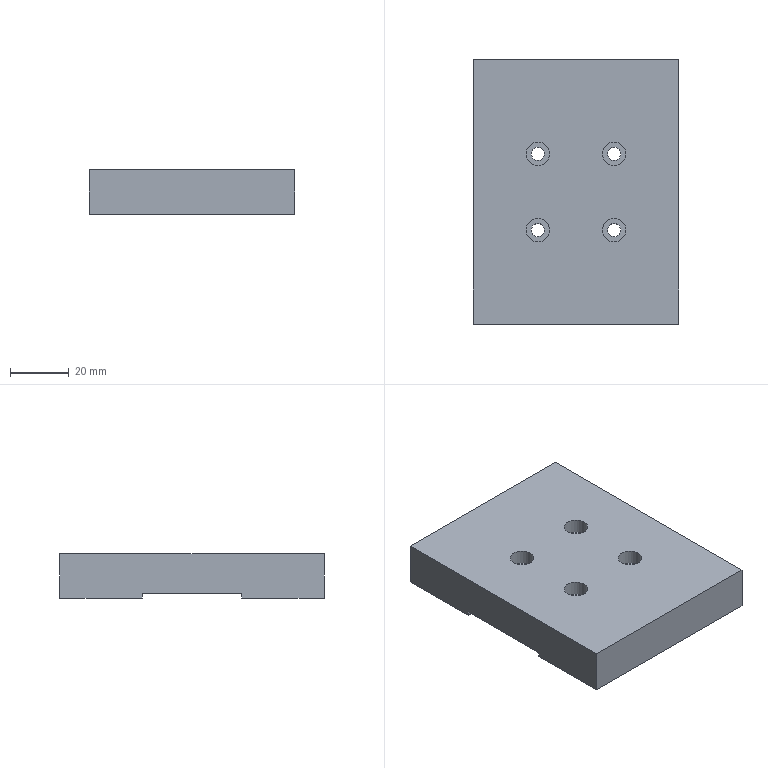Part | STEP file | Tube necking machine_id586_x_t | 1 solid | 22 faces | box 70 x 90 x 15 mm | volume 89384 mm3 | plane 14 | cylinder 8 | commonest cylinder face diameters 4.5 x4 8 x4
STEP:
#1=CARTESIAN_POINT('',(0.,0.,0.));
#2=DIRECTION('',(0.,0.,1.));
#3=DIRECTION('',(1.,0.,0.));
#4=AXIS2_PLACEMENT_3D('',#1,#2,#3);
#5=CARTESIAN_POINT('',(279.5,37.,156.));
#6=VERTEX_POINT('',#5);
#7=CARTESIAN_POINT('',(283.5,37.,156.));
#8=DIRECTION('',(0.,0.,-1.));
#9=DIRECTION('',(-1.,0.,0.));
#10=AXIS2_PLACEMENT_3D('',#7,#8,#9);
#11=CIRCLE('',#10,4.);
#12=CARTESIAN_POINT('',(8.,0.,156.));
#13=DIRECTION('',(0.,0.,-1.));
#14=DIRECTION('',(-1.,0.,0.));
#15=AXIS2_PLACEMENT_3D('',#12,#13,#14);
#16=PLANE('',#15);
#17=CARTESIAN_POINT('',(-275.5,37.));
#18=DIRECTION('',(1.,0.));
#19=AXIS2_PLACEMENT_2D('',#17,#18);
#20=CIRCLE('',#19,4.);
#21=(GEOMETRIC_REPRESENTATION_CONTEXT(2)PARAMETRIC_REPRESENTATION_CONTEXT()REPRESENTATION_CONTEXT('',''));
#22=DEFINITIONAL_REPRESENTATION('',(#20),#21);
#23=PCURVE('',#16,#22);
#24=CARTESIAN_POINT('',(283.5,37.,156.));
#25=DIRECTION('',(0.,0.,-1.));
#26=DIRECTION('',(-1.,0.,0.));
#27=AXIS2_PLACEMENT_3D('',#24,#25,#26);
#28=CYLINDRICAL_SURFACE('',#27,4.);
#29=CARTESIAN_POINT('',(0.,0.));
#30=DIRECTION('',(1.,0.));
#31=VECTOR('',#30,1.);
#32=LINE('',#29,#31);
#33=(GEOMETRIC_REPRESENTATION_CONTEXT(2)PARAMETRIC_REPRESENTATION_CONTEXT()REPRESENTATION_CONTEXT('',''));
#34=DEFINITIONAL_REPRESENTATION('',(#32),#33);
#35=PCURVE('',#28,#34);
#36=SURFACE_CURVE('',#11,(#23,#35),.PCURVE_S1.);
#37=EDGE_CURVE('',#6,#6,#36,.T.);
#38=ORIENTED_EDGE('',*,*,#37,.T.);
#39=EDGE_LOOP('',(#38));
#40=FACE_BOUND('',#39,.T.);
#41=CARTESIAN_POINT('',(253.5,37.,156.));
#42=VERTEX_POINT('',#41);
#43=CARTESIAN_POINT('',(257.5,37.,156.));
#44=DIRECTION('',(0.,0.,-1.));
#45=DIRECTION('',(-1.,0.,0.));
#46=AXIS2_PLACEMENT_3D('',#43,#44,#45);
#47=CIRCLE('',#46,4.);
#48=CARTESIAN_POINT('',(-249.5,37.));
#49=DIRECTION('',(1.,0.));
#50=AXIS2_PLACEMENT_2D('',#48,#49);
#51=CIRCLE('',#50,4.);
#52=(GEOMETRIC_REPRESENTATION_CONTEXT(2)PARAMETRIC_REPRESENTATION_CONTEXT()REPRESENTATION_CONTEXT('',''));
#53=DEFINITIONAL_REPRESENTATION('',(#51),#52);
#54=PCURVE('',#16,#53);
#55=CARTESIAN_POINT('',(257.5,37.,156.));
#56=DIRECTION('',(0.,0.,-1.));
#57=DIRECTION('',(-1.,0.,0.));
#58=AXIS2_PLACEMENT_3D('',#55,#56,#57);
#59=CYLINDRICAL_SURFACE('',#58,4.);
#60=CARTESIAN_POINT('',(0.,0.));
#61=DIRECTION('',(1.,0.));
#62=VECTOR('',#61,1.);
#63=LINE('',#60,#62);
#64=(GEOMETRIC_REPRESENTATION_CONTEXT(2)PARAMETRIC_REPRESENTATION_CONTEXT()REPRESENTATION_CONTEXT('',''));
#65=DEFINITIONAL_REPRESENTATION('',(#63),#64);
#66=PCURVE('',#59,#65);
#67=SURFACE_CURVE('',#47,(#54,#66),.PCURVE_S1.);
#68=EDGE_CURVE('',#42,#42,#67,.T.);
#69=ORIENTED_EDGE('',*,*,#68,.T.);
#70=EDGE_LOOP('',(#69));
#71=FACE_BOUND('',#70,.T.);
#72=CARTESIAN_POINT('',(279.5,63.,156.));
#73=VERTEX_POINT('',#72);
#74=CARTESIAN_POINT('',(283.5,63.,156.));
#75=DIRECTION('',(0.,0.,-1.));
#76=DIRECTION('',(-1.,0.,0.));
#77=AXIS2_PLACEMENT_3D('',#74,#75,#76);
#78=CIRCLE('',#77,4.);
#79=CARTESIAN_POINT('',(-275.5,63.));
#80=DIRECTION('',(1.,0.));
#81=AXIS2_PLACEMENT_2D('',#79,#80);
#82=CIRCLE('',#81,4.);
#83=(GEOMETRIC_REPRESENTATION_CONTEXT(2)PARAMETRIC_REPRESENTATION_CONTEXT()REPRESENTATION_CONTEXT('',''));
#84=DEFINITIONAL_REPRESENTATION('',(#82),#83);
#85=PCURVE('',#16,#84);
#86=CARTESIAN_POINT('',(283.5,63.,156.));
#87=DIRECTION('',(0.,0.,-1.));
#88=DIRECTION('',(-1.,0.,0.));
#89=AXIS2_PLACEMENT_3D('',#86,#87,#88);
#90=CYLINDRICAL_SURFACE('',#89,4.);
#91=CARTESIAN_POINT('',(0.,0.));
#92=DIRECTION('',(1.,0.));
#93=VECTOR('',#92,1.);
#94=LINE('',#91,#93);
#95=(GEOMETRIC_REPRESENTATION_CONTEXT(2)PARAMETRIC_REPRESENTATION_CONTEXT()REPRESENTATION_CONTEXT('',''));
#96=DEFINITIONAL_REPRESENTATION('',(#94),#95);
#97=PCURVE('',#90,#96);
#98=SURFACE_CURVE('',#78,(#85,#97),.PCURVE_S1.);
#99=EDGE_CURVE('',#73,#73,#98,.T.);
#100=ORIENTED_EDGE('',*,*,#99,.T.);
#101=EDGE_LOOP('',(#100));
#102=FACE_BOUND('',#101,.T.);
#103=CARTESIAN_POINT('',(253.5,63.,156.));
#104=VERTEX_POINT('',#103);
#105=CARTESIAN_POINT('',(257.5,63.,156.));
#106=DIRECTION('',(0.,0.,-1.));
#107=DIRECTION('',(-1.,0.,0.));
#108=AXIS2_PLACEMENT_3D('',#105,#106,#107);
#109=CIRCLE('',#108,4.);
#110=CARTESIAN_POINT('',(-249.5,63.));
#111=DIRECTION('',(1.,0.));
#112=AXIS2_PLACEMENT_2D('',#110,#111);
#113=CIRCLE('',#112,4.);
#114=(GEOMETRIC_REPRESENTATION_CONTEXT(2)PARAMETRIC_REPRESENTATION_CONTEXT()REPRESENTATION_CONTEXT('',''));
#115=DEFINITIONAL_REPRESENTATION('',(#113),#114);
#116=PCURVE('',#16,#115);
#117=CARTESIAN_POINT('',(257.5,63.,156.));
#118=DIRECTION('',(0.,0.,-1.));
#119=DIRECTION('',(-1.,0.,0.));
#120=AXIS2_PLACEMENT_3D('',#117,#118,#119);
#121=CYLINDRICAL_SURFACE('',#120,4.);
#122=CARTESIAN_POINT('',(0.,0.));
#123=DIRECTION('',(1.,0.));
#124=VECTOR('',#123,1.);
#125=LINE('',#122,#124);
#126=(GEOMETRIC_REPRESENTATION_CONTEXT(2)PARAMETRIC_REPRESENTATION_CONTEXT()REPRESENTATION_CONTEXT('',''));
#127=DEFINITIONAL_REPRESENTATION('',(#125),#126);
#128=PCURVE('',#121,#127);
#129=SURFACE_CURVE('',#109,(#116,#128),.PCURVE_S1.);
#130=EDGE_CURVE('',#104,#104,#129,.T.);
#131=ORIENTED_EDGE('',*,*,#130,.T.);
#132=EDGE_LOOP('',(#131));
#133=FACE_BOUND('',#132,.T.);
#134=CARTESIAN_POINT('',(305.5,95.,156.));
#135=VERTEX_POINT('',#134);
#136=CARTESIAN_POINT('',(305.5,5.,156.));
#137=VERTEX_POINT('',#136);
#138=CARTESIAN_POINT('',(305.5,95.,156.));
#139=DIRECTION('',(0.,-1.,0.));
#140=VECTOR('',#139,1.);
#141=LINE('',#138,#140);
#142=CARTESIAN_POINT('',(-297.5,95.));
#143=DIRECTION('',(0.,-1.));
#144=VECTOR('',#143,1.);
#145=LINE('',#142,#144);
#146=(GEOMETRIC_REPRESENTATION_CONTEXT(2)PARAMETRIC_REPRESENTATION_CONTEXT()REPRESENTATION_CONTEXT('',''));
#147=DEFINITIONAL_REPRESENTATION('',(#145),#146);
#148=PCURVE('',#16,#147);
#149=CARTESIAN_POINT('',(305.5,95.,141.));
#150=DIRECTION('',(-1.,0.,0.));
#151=DIRECTION('',(0.,0.,1.));
#152=AXIS2_PLACEMENT_3D('',#149,#150,#151);
#153=PLANE('',#152);
#154=CARTESIAN_POINT('',(15.,0.));
#155=DIRECTION('',(0.,-1.));
#156=VECTOR('',#155,1.);
#157=LINE('',#154,#156);
#158=(GEOMETRIC_REPRESENTATION_CONTEXT(2)PARAMETRIC_REPRESENTATION_CONTEXT()REPRESENTATION_CONTEXT('',''));
#159=DEFINITIONAL_REPRESENTATION('',(#157),#158);
#160=PCURVE('',#153,#159);
#161=SURFACE_CURVE('',#141,(#148,#160),.PCURVE_S1.);
#162=EDGE_CURVE('',#135,#137,#161,.T.);
#163=ORIENTED_EDGE('',*,*,#162,.F.);
#164=CARTESIAN_POINT('',(235.5,95.,156.));
#165=VERTEX_POINT('',#164);
#166=CARTESIAN_POINT('',(235.5,95.,156.));
#167=DIRECTION('',(1.,0.,0.));
#168=VECTOR('',#167,1.);
#169=LINE('',#166,#168);
#170=CARTESIAN_POINT('',(-227.5,95.));
#171=DIRECTION('',(-1.,0.));
#172=VECTOR('',#171,1.);
#173=LINE('',#170,#172);
#174=(GEOMETRIC_REPRESENTATION_CONTEXT(2)PARAMETRIC_REPRESENTATION_CONTEXT()REPRESENTATION_CONTEXT('',''));
#175=DEFINITIONAL_REPRESENTATION('',(#173),#174);
#176=PCURVE('',#16,#175);
#177=CARTESIAN_POINT('',(235.5,95.,141.));
#178=DIRECTION('',(0.,-1.,0.));
#179=DIRECTION('',(0.,0.,-1.));
#180=AXIS2_PLACEMENT_3D('',#177,#178,#179);
#181=PLANE('',#180);
#182=CARTESIAN_POINT('',(-15.,0.));
#183=DIRECTION('',(0.,1.));
#184=VECTOR('',#183,1.);
#185=LINE('',#182,#184);
#186=(GEOMETRIC_REPRESENTATION_CONTEXT(2)PARAMETRIC_REPRESENTATION_CONTEXT()REPRESENTATION_CONTEXT('',''));
#187=DEFINITIONAL_REPRESENTATION('',(#185),#186);
#188=PCURVE('',#181,#187);
#189=SURFACE_CURVE('',#169,(#176,#188),.PCURVE_S1.);
#190=EDGE_CURVE('',#165,#135,#189,.T.);
#191=ORIENTED_EDGE('',*,*,#190,.F.);
#192=CARTESIAN_POINT('',(235.5,5.,156.));
#193=VERTEX_POINT('',#192);
#194=CARTESIAN_POINT('',(235.5,5.,156.));
#195=DIRECTION('',(0.,1.,0.));
#196=VECTOR('',#195,1.);
#197=LINE('',#194,#196);
#198=CARTESIAN_POINT('',(-227.5,5.));
#199=DIRECTION('',(0.,1.));
#200=VECTOR('',#199,1.);
#201=LINE('',#198,#200);
#202=(GEOMETRIC_REPRESENTATION_CONTEXT(2)PARAMETRIC_REPRESENTATION_CONTEXT()REPRESENTATION_CONTEXT('',''));
#203=DEFINITIONAL_REPRESENTATION('',(#201),#202);
#204=PCURVE('',#16,#203);
#205=CARTESIAN_POINT('',(235.5,5.,141.));
#206=DIRECTION('',(1.,0.,0.));
#207=DIRECTION('',(0.,0.,-1.));
#208=AXIS2_PLACEMENT_3D('',#205,#206,#207);
#209=PLANE('',#208);
#210=CARTESIAN_POINT('',(-15.,0.));
#211=DIRECTION('',(0.,1.));
#212=VECTOR('',#211,1.);
#213=LINE('',#210,#212);
#214=(GEOMETRIC_REPRESENTATION_CONTEXT(2)PARAMETRIC_REPRESENTATION_CONTEXT()REPRESENTATION_CONTEXT('',''));
#215=DEFINITIONAL_REPRESENTATION('',(#213),#214);
#216=PCURVE('',#209,#215);
#217=SURFACE_CURVE('',#197,(#204,#216),.PCURVE_S1.);
#218=EDGE_CURVE('',#193,#165,#217,.T.);
#219=ORIENTED_EDGE('',*,*,#218,.F.);
#220=CARTESIAN_POINT('',(250.5,5.,156.));
#221=DIRECTION('',(-1.,0.,0.));
#222=VECTOR('',#221,1.);
#223=LINE('',#220,#222);
#224=CARTESIAN_POINT('',(-242.5,5.));
#225=DIRECTION('',(1.,0.));
#226=VECTOR('',#225,1.);
#227=LINE('',#224,#226);
#228=(GEOMETRIC_REPRESENTATION_CONTEXT(2)PARAMETRIC_REPRESENTATION_CONTEXT()REPRESENTATION_CONTEXT('',''));
#229=DEFINITIONAL_REPRESENTATION('',(#227),#228);
#230=PCURVE('',#16,#229);
#231=CARTESIAN_POINT('',(250.5,5.,141.));
#232=DIRECTION('',(0.,1.,0.));
#233=DIRECTION('',(0.,0.,1.));
#234=AXIS2_PLACEMENT_3D('',#231,#232,#233);
#235=PLANE('',#234);
#236=CARTESIAN_POINT('',(15.,0.));
#237=DIRECTION('',(0.,-1.));
#238=VECTOR('',#237,1.);
#239=LINE('',#236,#238);
#240=(GEOMETRIC_REPRESENTATION_CONTEXT(2)PARAMETRIC_REPRESENTATION_CONTEXT()REPRESENTATION_CONTEXT('',''));
#241=DEFINITIONAL_REPRESENTATION('',(#239),#240);
#242=PCURVE('',#235,#241);
#243=SURFACE_CURVE('',#223,(#230,#242),.PCURVE_S1.);
#244=EDGE_CURVE('',#137,#193,#243,.T.);
#245=ORIENTED_EDGE('',*,*,#244,.F.);
#246=EDGE_LOOP('',(#163,#191,#219,#245));
#247=FACE_BOUND('',#246,.T.);
#248=ADVANCED_FACE('',(#40,#71,#102,#133,#247),#16,.F.);
#249=CARTESIAN_POINT('',(281.25,37.,142.5));
#250=VERTEX_POINT('',#249);
#251=CARTESIAN_POINT('',(283.5,37.,142.5));
#252=DIRECTION('',(0.,0.,-1.));
#253=DIRECTION('',(-1.,0.,0.));
#254=AXIS2_PLACEMENT_3D('',#251,#252,#253);
#255=CIRCLE('',#254,2.25);
#256=CARTESIAN_POINT('',(315.2,33.,142.5));
#257=DIRECTION('',(0.,0.,-1.));
#258=DIRECTION('',(1.,0.,0.));
#259=AXIS2_PLACEMENT_3D('',#256,#257,#258);
#260=PLANE('',#259);
#261=CARTESIAN_POINT('',(-31.7,-4.));
#262=DIRECTION('',(-1.,0.));
#263=AXIS2_PLACEMENT_2D('',#261,#262);
#264=CIRCLE('',#263,2.25);
#265=(GEOMETRIC_REPRESENTATION_CONTEXT(2)PARAMETRIC_REPRESENTATION_CONTEXT()REPRESENTATION_CONTEXT('',''));
#266=DEFINITIONAL_REPRESENTATION('',(#264),#265);
#267=PCURVE('',#260,#266);
#268=CARTESIAN_POINT('',(283.5,37.,136.));
#269=DIRECTION('',(0.,0.,-1.));
#270=DIRECTION('',(-1.,0.,0.));
#271=AXIS2_PLACEMENT_3D('',#268,#269,#270);
#272=CYLINDRICAL_SURFACE('',#271,2.25);
#273=CARTESIAN_POINT('',(0.,-6.5));
#274=DIRECTION('',(1.,0.));
#275=VECTOR('',#274,1.);
#276=LINE('',#273,#275);
#277=(GEOMETRIC_REPRESENTATION_CONTEXT(2)PARAMETRIC_REPRESENTATION_CONTEXT()REPRESENTATION_CONTEXT('',''));
#278=DEFINITIONAL_REPRESENTATION('',(#276),#277);
#279=PCURVE('',#272,#278);
#280=SURFACE_CURVE('',#255,(#267,#279),.PCURVE_S1.);
#281=EDGE_CURVE('',#250,#250,#280,.T.);
#282=ORIENTED_EDGE('',*,*,#281,.F.);
#283=EDGE_LOOP('',(#282));
#284=FACE_BOUND('',#283,.T.);
#285=CARTESIAN_POINT('',(255.25,37.,142.5));
#286=VERTEX_POINT('',#285);
#287=CARTESIAN_POINT('',(257.5,37.,142.5));
#288=DIRECTION('',(0.,0.,-1.));
#289=DIRECTION('',(-1.,0.,0.));
#290=AXIS2_PLACEMENT_3D('',#287,#288,#289);
#291=CIRCLE('',#290,2.25);
#292=CARTESIAN_POINT('',(-57.7,-4.));
#293=DIRECTION('',(-1.,0.));
#294=AXIS2_PLACEMENT_2D('',#292,#293);
#295=CIRCLE('',#294,2.25);
#296=(GEOMETRIC_REPRESENTATION_CONTEXT(2)PARAMETRIC_REPRESENTATION_CONTEXT()REPRESENTATION_CONTEXT('',''));
#297=DEFINITIONAL_REPRESENTATION('',(#295),#296);
#298=PCURVE('',#260,#297);
#299=CARTESIAN_POINT('',(257.5,37.,136.));
#300=DIRECTION('',(0.,0.,-1.));
#301=DIRECTION('',(-1.,0.,0.));
#302=AXIS2_PLACEMENT_3D('',#299,#300,#301);
#303=CYLINDRICAL_SURFACE('',#302,2.25);
#304=CARTESIAN_POINT('',(0.,-6.5));
#305=DIRECTION('',(1.,0.));
#306=VECTOR('',#305,1.);
#307=LINE('',#304,#306);
#308=(GEOMETRIC_REPRESENTATION_CONTEXT(2)PARAMETRIC_REPRESENTATION_CONTEXT()REPRESENTATION_CONTEXT('',''));
#309=DEFINITIONAL_REPRESENTATION('',(#307),#308);
#310=PCURVE('',#303,#309);
#311=SURFACE_CURVE('',#291,(#298,#310),.PCURVE_S1.);
#312=EDGE_CURVE('',#286,#286,#311,.T.);
#313=ORIENTED_EDGE('',*,*,#312,.F.);
#314=EDGE_LOOP('',(#313));
#315=FACE_BOUND('',#314,.T.);
#316=CARTESIAN_POINT('',(281.25,63.,142.5));
#317=VERTEX_POINT('',#316);
#318=CARTESIAN_POINT('',(283.5,63.,142.5));
#319=DIRECTION('',(0.,0.,-1.));
#320=DIRECTION('',(-1.,0.,0.));
#321=AXIS2_PLACEMENT_3D('',#318,#319,#320);
#322=CIRCLE('',#321,2.25);
#323=CARTESIAN_POINT('',(-31.7,-30.));
#324=DIRECTION('',(-1.,0.));
#325=AXIS2_PLACEMENT_2D('',#323,#324);
#326=CIRCLE('',#325,2.25);
#327=(GEOMETRIC_REPRESENTATION_CONTEXT(2)PARAMETRIC_REPRESENTATION_CONTEXT()REPRESENTATION_CONTEXT('',''));
#328=DEFINITIONAL_REPRESENTATION('',(#326),#327);
#329=PCURVE('',#260,#328);
#330=CARTESIAN_POINT('',(283.5,63.,136.));
#331=DIRECTION('',(0.,0.,-1.));
#332=DIRECTION('',(-1.,0.,0.));
#333=AXIS2_PLACEMENT_3D('',#330,#331,#332);
#334=CYLINDRICAL_SURFACE('',#333,2.25);
#335=CARTESIAN_POINT('',(0.,-6.5));
#336=DIRECTION('',(1.,0.));
#337=VECTOR('',#336,1.);
#338=LINE('',#335,#337);
#339=(GEOMETRIC_REPRESENTATION_CONTEXT(2)PARAMETRIC_REPRESENTATION_CONTEXT()REPRESENTATION_CONTEXT('',''));
#340=DEFINITIONAL_REPRESENTATION('',(#338),#339);
#341=PCURVE('',#334,#340);
#342=SURFACE_CURVE('',#322,(#329,#341),.PCURVE_S1.);
#343=EDGE_CURVE('',#317,#317,#342,.T.);
#344=ORIENTED_EDGE('',*,*,#343,.F.);
#345=EDGE_LOOP('',(#344));
#346=FACE_BOUND('',#345,.T.);
#347=CARTESIAN_POINT('',(255.25,63.,142.5));
#348=VERTEX_POINT('',#347);
#349=CARTESIAN_POINT('',(257.5,63.,142.5));
#350=DIRECTION('',(0.,0.,-1.));
#351=DIRECTION('',(-1.,0.,0.));
#352=AXIS2_PLACEMENT_3D('',#349,#350,#351);
#353=CIRCLE('',#352,2.25);
#354=CARTESIAN_POINT('',(-57.7,-30.));
#355=DIRECTION('',(-1.,0.));
#356=AXIS2_PLACEMENT_2D('',#354,#355);
#357=CIRCLE('',#356,2.25);
#358=(GEOMETRIC_REPRESENTATION_CONTEXT(2)PARAMETRIC_REPRESENTATION_CONTEXT()REPRESENTATION_CONTEXT('',''));
#359=DEFINITIONAL_REPRESENTATION('',(#357),#358);
#360=PCURVE('',#260,#359);
#361=CARTESIAN_POINT('',(257.5,63.,136.));
#362=DIRECTION('',(0.,0.,-1.));
#363=DIRECTION('',(-1.,0.,0.));
#364=AXIS2_PLACEMENT_3D('',#361,#362,#363);
#365=CYLINDRICAL_SURFACE('',#364,2.25);
#366=CARTESIAN_POINT('',(0.,-6.5));
#367=DIRECTION('',(1.,0.));
#368=VECTOR('',#367,1.);
#369=LINE('',#366,#368);
#370=(GEOMETRIC_REPRESENTATION_CONTEXT(2)PARAMETRIC_REPRESENTATION_CONTEXT()REPRESENTATION_CONTEXT('',''));
#371=DEFINITIONAL_REPRESENTATION('',(#369),#370);
#372=PCURVE('',#365,#371);
#373=SURFACE_CURVE('',#353,(#360,#372),.PCURVE_S1.);
#374=EDGE_CURVE('',#348,#348,#373,.T.);
#375=ORIENTED_EDGE('',*,*,#374,.F.);
#376=EDGE_LOOP('',(#375));
#377=FACE_BOUND('',#376,.T.);
#378=CARTESIAN_POINT('',(305.5,33.,142.5));
#379=VERTEX_POINT('',#378);
#380=CARTESIAN_POINT('',(235.5,33.,142.5));
#381=VERTEX_POINT('',#380);
#382=CARTESIAN_POINT('',(315.2,33.,142.5));
#383=DIRECTION('',(-1.,0.,0.));
#384=VECTOR('',#383,1.);
#385=LINE('',#382,#384);
#386=CARTESIAN_POINT('',(0.,0.));
#387=DIRECTION('',(-1.,0.));
#388=VECTOR('',#387,1.);
#389=LINE('',#386,#388);
#390=(GEOMETRIC_REPRESENTATION_CONTEXT(2)PARAMETRIC_REPRESENTATION_CONTEXT()REPRESENTATION_CONTEXT('',''));
#391=DEFINITIONAL_REPRESENTATION('',(#389),#390);
#392=PCURVE('',#260,#391);
#393=CARTESIAN_POINT('',(315.2,33.,116.));
#394=DIRECTION('',(0.,1.,0.));
#395=DIRECTION('',(0.,0.,1.));
#396=AXIS2_PLACEMENT_3D('',#393,#394,#395);
#397=PLANE('',#396);
#398=CARTESIAN_POINT('',(26.5,0.));
#399=DIRECTION('',(0.,-1.));
#400=VECTOR('',#399,1.);
#401=LINE('',#398,#400);
#402=(GEOMETRIC_REPRESENTATION_CONTEXT(2)PARAMETRIC_REPRESENTATION_CONTEXT()REPRESENTATION_CONTEXT('',''));
#403=DEFINITIONAL_REPRESENTATION('',(#401),#402);
#404=PCURVE('',#397,#403);
#405=SURFACE_CURVE('',#385,(#392,#404),.PCURVE_S1.);
#406=EDGE_CURVE('',#379,#381,#405,.T.);
#407=ORIENTED_EDGE('',*,*,#406,.T.);
#408=CARTESIAN_POINT('',(235.5,67.,142.5));
#409=VERTEX_POINT('',#408);
#410=CARTESIAN_POINT('',(235.5,5.,142.5));
#411=DIRECTION('',(0.,1.,0.));
#412=VECTOR('',#411,1.);
#413=LINE('',#410,#412);
#414=CARTESIAN_POINT('',(-79.7,28.));
#415=DIRECTION('',(0.,-1.));
#416=VECTOR('',#415,1.);
#417=LINE('',#414,#416);
#418=(GEOMETRIC_REPRESENTATION_CONTEXT(2)PARAMETRIC_REPRESENTATION_CONTEXT()REPRESENTATION_CONTEXT('',''));
#419=DEFINITIONAL_REPRESENTATION('',(#417),#418);
#420=PCURVE('',#260,#419);
#421=CARTESIAN_POINT('',(-1.5,0.));
#422=DIRECTION('',(0.,1.));
#423=VECTOR('',#422,1.);
#424=LINE('',#421,#423);
#425=(GEOMETRIC_REPRESENTATION_CONTEXT(2)PARAMETRIC_REPRESENTATION_CONTEXT()REPRESENTATION_CONTEXT('',''));
#426=DEFINITIONAL_REPRESENTATION('',(#424),#425);
#427=PCURVE('',#209,#426);
#428=SURFACE_CURVE('',#413,(#420,#427),.PCURVE_S1.);
#429=EDGE_CURVE('',#381,#409,#428,.T.);
#430=ORIENTED_EDGE('',*,*,#429,.T.);
#431=CARTESIAN_POINT('',(305.5,67.,142.5));
#432=VERTEX_POINT('',#431);
#433=CARTESIAN_POINT('',(315.2,67.,142.5));
#434=DIRECTION('',(-1.,0.,0.));
#435=VECTOR('',#434,1.);
#436=LINE('',#433,#435);
#437=CARTESIAN_POINT('',(0.,-34.));
#438=DIRECTION('',(-1.,0.));
#439=VECTOR('',#438,1.);
#440=LINE('',#437,#439);
#441=(GEOMETRIC_REPRESENTATION_CONTEXT(2)PARAMETRIC_REPRESENTATION_CONTEXT()REPRESENTATION_CONTEXT('',''));
#442=DEFINITIONAL_REPRESENTATION('',(#440),#441);
#443=PCURVE('',#260,#442);
#444=CARTESIAN_POINT('',(315.2,67.,144.));
#445=DIRECTION('',(0.,-1.,0.));
#446=DIRECTION('',(0.,0.,-1.));
#447=AXIS2_PLACEMENT_3D('',#444,#445,#446);
#448=PLANE('',#447);
#449=CARTESIAN_POINT('',(1.5,0.));
#450=DIRECTION('',(0.,-1.));
#451=VECTOR('',#450,1.);
#452=LINE('',#449,#451);
#453=(GEOMETRIC_REPRESENTATION_CONTEXT(2)PARAMETRIC_REPRESENTATION_CONTEXT()REPRESENTATION_CONTEXT('',''));
#454=DEFINITIONAL_REPRESENTATION('',(#452),#453);
#455=PCURVE('',#448,#454);
#456=SURFACE_CURVE('',#436,(#443,#455),.PCURVE_S1.);
#457=EDGE_CURVE('',#432,#409,#456,.T.);
#458=ORIENTED_EDGE('',*,*,#457,.F.);
#459=CARTESIAN_POINT('',(305.5,33.,142.5));
#460=DIRECTION('',(0.,1.,0.));
#461=VECTOR('',#460,1.);
#462=LINE('',#459,#461);
#463=CARTESIAN_POINT('',(-9.7,0.));
#464=DIRECTION('',(0.,-1.));
#465=VECTOR('',#464,1.);
#466=LINE('',#463,#465);
#467=(GEOMETRIC_REPRESENTATION_CONTEXT(2)PARAMETRIC_REPRESENTATION_CONTEXT()REPRESENTATION_CONTEXT('',''));
#468=DEFINITIONAL_REPRESENTATION('',(#466),#467);
#469=PCURVE('',#260,#468);
#470=CARTESIAN_POINT('',(1.5,-62.));
#471=DIRECTION('',(0.,1.));
#472=VECTOR('',#471,1.);
#473=LINE('',#470,#472);
#474=(GEOMETRIC_REPRESENTATION_CONTEXT(2)PARAMETRIC_REPRESENTATION_CONTEXT()REPRESENTATION_CONTEXT('',''));
#475=DEFINITIONAL_REPRESENTATION('',(#473),#474);
#476=PCURVE('',#153,#475);
#477=SURFACE_CURVE('',#462,(#469,#476),.PCURVE_S1.);
#478=EDGE_CURVE('',#379,#432,#477,.T.);
#479=ORIENTED_EDGE('',*,*,#478,.F.);
#480=EDGE_LOOP('',(#407,#430,#458,#479));
#481=FACE_BOUND('',#480,.T.);
#482=ADVANCED_FACE('',(#284,#315,#346,#377,#481),#260,.T.);
#483=CARTESIAN_POINT('',(235.5,33.,141.));
#484=VERTEX_POINT('',#483);
#485=CARTESIAN_POINT('',(305.5,33.,141.));
#486=VERTEX_POINT('',#485);
#487=CARTESIAN_POINT('',(8.,33.,141.));
#488=DIRECTION('',(1.,0.,0.));
#489=VECTOR('',#488,1.);
#490=LINE('',#487,#489);
#491=CARTESIAN_POINT('',(8.,0.,141.));
#492=DIRECTION('',(0.,0.,-1.));
#493=DIRECTION('',(-1.,0.,0.));
#494=AXIS2_PLACEMENT_3D('',#491,#492,#493);
#495=PLANE('',#494);
#496=CARTESIAN_POINT('',(0.,33.));
#497=DIRECTION('',(-1.,0.));
#498=VECTOR('',#497,1.);
#499=LINE('',#496,#498);
#500=(GEOMETRIC_REPRESENTATION_CONTEXT(2)PARAMETRIC_REPRESENTATION_CONTEXT()REPRESENTATION_CONTEXT('',''));
#501=DEFINITIONAL_REPRESENTATION('',(#499),#500);
#502=PCURVE('',#495,#501);
#503=CARTESIAN_POINT('',(25.,-307.2));
#504=DIRECTION('',(0.,1.));
#505=VECTOR('',#504,1.);
#506=LINE('',#503,#505);
#507=(GEOMETRIC_REPRESENTATION_CONTEXT(2)PARAMETRIC_REPRESENTATION_CONTEXT()REPRESENTATION_CONTEXT('',''));
#508=DEFINITIONAL_REPRESENTATION('',(#506),#507);
#509=PCURVE('',#397,#508);
#510=SURFACE_CURVE('',#490,(#502,#509),.PCURVE_S1.);
#511=EDGE_CURVE('',#484,#486,#510,.T.);
#512=ORIENTED_EDGE('',*,*,#511,.T.);
#513=CARTESIAN_POINT('',(305.5,5.,141.));
#514=VERTEX_POINT('',#513);
#515=CARTESIAN_POINT('',(305.5,95.,141.));
#516=DIRECTION('',(0.,-1.,0.));
#517=VECTOR('',#516,1.);
#518=LINE('',#515,#517);
#519=CARTESIAN_POINT('',(-297.5,95.));
#520=DIRECTION('',(0.,-1.));
#521=VECTOR('',#520,1.);
#522=LINE('',#519,#521);
#523=(GEOMETRIC_REPRESENTATION_CONTEXT(2)PARAMETRIC_REPRESENTATION_CONTEXT()REPRESENTATION_CONTEXT('',''));
#524=DEFINITIONAL_REPRESENTATION('',(#522),#523);
#525=PCURVE('',#495,#524);
#526=CARTESIAN_POINT('',(0.,0.));
#527=DIRECTION('',(0.,-1.));
#528=VECTOR('',#527,1.);
#529=LINE('',#526,#528);
#530=(GEOMETRIC_REPRESENTATION_CONTEXT(2)PARAMETRIC_REPRESENTATION_CONTEXT()REPRESENTATION_CONTEXT('',''));
#531=DEFINITIONAL_REPRESENTATION('',(#529),#530);
#532=PCURVE('',#153,#531);
#533=SURFACE_CURVE('',#518,(#525,#532),.PCURVE_S1.);
#534=EDGE_CURVE('',#486,#514,#533,.T.);
#535=ORIENTED_EDGE('',*,*,#534,.T.);
#536=CARTESIAN_POINT('',(235.5,5.,141.));
#537=VERTEX_POINT('',#536);
#538=CARTESIAN_POINT('',(305.5,5.,141.));
#539=DIRECTION('',(-1.,0.,0.));
#540=VECTOR('',#539,1.);
#541=LINE('',#538,#540);
#542=CARTESIAN_POINT('',(-297.5,5.));
#543=DIRECTION('',(1.,0.));
#544=VECTOR('',#543,1.);
#545=LINE('',#542,#544);
#546=(GEOMETRIC_REPRESENTATION_CONTEXT(2)PARAMETRIC_REPRESENTATION_CONTEXT()REPRESENTATION_CONTEXT('',''));
#547=DEFINITIONAL_REPRESENTATION('',(#545),#546);
#548=PCURVE('',#495,#547);
#549=CARTESIAN_POINT('',(0.,55.));
#550=DIRECTION('',(0.,-1.));
#551=VECTOR('',#550,1.);
#552=LINE('',#549,#551);
#553=(GEOMETRIC_REPRESENTATION_CONTEXT(2)PARAMETRIC_REPRESENTATION_CONTEXT()REPRESENTATION_CONTEXT('',''));
#554=DEFINITIONAL_REPRESENTATION('',(#552),#553);
#555=PCURVE('',#235,#554);
#556=SURFACE_CURVE('',#541,(#548,#555),.PCURVE_S1.);
#557=EDGE_CURVE('',#514,#537,#556,.T.);
#558=ORIENTED_EDGE('',*,*,#557,.T.);
#559=CARTESIAN_POINT('',(235.5,5.,141.));
#560=DIRECTION('',(0.,1.,0.));
#561=VECTOR('',#560,1.);
#562=LINE('',#559,#561);
#563=CARTESIAN_POINT('',(-227.5,5.));
#564=DIRECTION('',(0.,1.));
#565=VECTOR('',#564,1.);
#566=LINE('',#563,#565);
#567=(GEOMETRIC_REPRESENTATION_CONTEXT(2)PARAMETRIC_REPRESENTATION_CONTEXT()REPRESENTATION_CONTEXT('',''));
#568=DEFINITIONAL_REPRESENTATION('',(#566),#567);
#569=PCURVE('',#495,#568);
#570=CARTESIAN_POINT('',(0.,0.));
#571=DIRECTION('',(0.,1.));
#572=VECTOR('',#571,1.);
#573=LINE('',#570,#572);
#574=(GEOMETRIC_REPRESENTATION_CONTEXT(2)PARAMETRIC_REPRESENTATION_CONTEXT()REPRESENTATION_CONTEXT('',''));
#575=DEFINITIONAL_REPRESENTATION('',(#573),#574);
#576=PCURVE('',#209,#575);
#577=SURFACE_CURVE('',#562,(#569,#576),.PCURVE_S1.);
#578=EDGE_CURVE('',#537,#484,#577,.T.);
#579=ORIENTED_EDGE('',*,*,#578,.T.);
#580=EDGE_LOOP('',(#512,#535,#558,#579));
#581=FACE_BOUND('',#580,.T.);
#582=ADVANCED_FACE('',(#581),#495,.T.);
#583=ORIENTED_EDGE('',*,*,#478,.T.);
#584=CARTESIAN_POINT('',(305.5,67.,141.));
#585=VERTEX_POINT('',#584);
#586=CARTESIAN_POINT('',(305.5,67.,141.));
#587=DIRECTION('',(0.,0.,1.));
#588=VECTOR('',#587,1.);
#589=LINE('',#586,#588);
#590=CARTESIAN_POINT('',(0.,-28.));
#591=DIRECTION('',(1.,0.));
#592=VECTOR('',#591,1.);
#593=LINE('',#590,#592);
#594=(GEOMETRIC_REPRESENTATION_CONTEXT(2)PARAMETRIC_REPRESENTATION_CONTEXT()REPRESENTATION_CONTEXT('',''));
#595=DEFINITIONAL_REPRESENTATION('',(#593),#594);
#596=PCURVE('',#153,#595);
#597=CARTESIAN_POINT('',(3.,-9.7));
#598=DIRECTION('',(-1.,0.));
#599=VECTOR('',#598,1.);
#600=LINE('',#597,#599);
#601=(GEOMETRIC_REPRESENTATION_CONTEXT(2)PARAMETRIC_REPRESENTATION_CONTEXT()REPRESENTATION_CONTEXT('',''));
#602=DEFINITIONAL_REPRESENTATION('',(#600),#601);
#603=PCURVE('',#448,#602);
#604=SURFACE_CURVE('',#589,(#596,#603),.PCURVE_S1.);
#605=EDGE_CURVE('',#585,#432,#604,.T.);
#606=ORIENTED_EDGE('',*,*,#605,.F.);
#607=CARTESIAN_POINT('',(305.5,95.,141.));
#608=VERTEX_POINT('',#607);
#609=CARTESIAN_POINT('',(305.5,95.,141.));
#610=DIRECTION('',(0.,-1.,0.));
#611=VECTOR('',#610,1.);
#612=LINE('',#609,#611);
#613=CARTESIAN_POINT('',(0.,0.));
#614=DIRECTION('',(0.,-1.));
#615=VECTOR('',#614,1.);
#616=LINE('',#613,#615);
#617=(GEOMETRIC_REPRESENTATION_CONTEXT(2)PARAMETRIC_REPRESENTATION_CONTEXT()REPRESENTATION_CONTEXT('',''));
#618=DEFINITIONAL_REPRESENTATION('',(#616),#617);
#619=PCURVE('',#153,#618);
#620=CARTESIAN_POINT('',(8.,0.,141.));
#621=DIRECTION('',(0.,0.,-1.));
#622=DIRECTION('',(-1.,0.,0.));
#623=AXIS2_PLACEMENT_3D('',#620,#621,#622);
#624=PLANE('',#623);
#625=CARTESIAN_POINT('',(-297.5,95.));
#626=DIRECTION('',(0.,-1.));
#627=VECTOR('',#626,1.);
#628=LINE('',#625,#627);
#629=(GEOMETRIC_REPRESENTATION_CONTEXT(2)PARAMETRIC_REPRESENTATION_CONTEXT()REPRESENTATION_CONTEXT('',''));
#630=DEFINITIONAL_REPRESENTATION('',(#628),#629);
#631=PCURVE('',#624,#630);
#632=SURFACE_CURVE('',#612,(#619,#631),.PCURVE_S1.);
#633=EDGE_CURVE('',#608,#585,#632,.T.);
#634=ORIENTED_EDGE('',*,*,#633,.F.);
#635=CARTESIAN_POINT('',(305.5,95.,141.));
#636=DIRECTION('',(0.,0.,1.));
#637=VECTOR('',#636,1.);
#638=LINE('',#635,#637);
#639=CARTESIAN_POINT('',(0.,0.));
#640=DIRECTION('',(1.,0.));
#641=VECTOR('',#640,1.);
#642=LINE('',#639,#641);
#643=(GEOMETRIC_REPRESENTATION_CONTEXT(2)PARAMETRIC_REPRESENTATION_CONTEXT()REPRESENTATION_CONTEXT('',''));
#644=DEFINITIONAL_REPRESENTATION('',(#642),#643);
#645=PCURVE('',#153,#644);
#646=CARTESIAN_POINT('',(0.,70.));
#647=DIRECTION('',(-1.,0.));
#648=VECTOR('',#647,1.);
#649=LINE('',#646,#648);
#650=(GEOMETRIC_REPRESENTATION_CONTEXT(2)PARAMETRIC_REPRESENTATION_CONTEXT()REPRESENTATION_CONTEXT('',''));
#651=DEFINITIONAL_REPRESENTATION('',(#649),#650);
#652=PCURVE('',#181,#651);
#653=SURFACE_CURVE('',#638,(#645,#652),.PCURVE_S1.);
#654=EDGE_CURVE('',#608,#135,#653,.T.);
#655=ORIENTED_EDGE('',*,*,#654,.T.);
#656=ORIENTED_EDGE('',*,*,#162,.T.);
#657=CARTESIAN_POINT('',(305.5,5.,141.));
#658=DIRECTION('',(0.,0.,1.));
#659=VECTOR('',#658,1.);
#660=LINE('',#657,#659);
#661=CARTESIAN_POINT('',(0.,-90.));
#662=DIRECTION('',(1.,0.));
#663=VECTOR('',#662,1.);
#664=LINE('',#661,#663);
#665=(GEOMETRIC_REPRESENTATION_CONTEXT(2)PARAMETRIC_REPRESENTATION_CONTEXT()REPRESENTATION_CONTEXT('',''));
#666=DEFINITIONAL_REPRESENTATION('',(#664),#665);
#667=PCURVE('',#153,#666);
#668=CARTESIAN_POINT('',(0.,55.));
#669=DIRECTION('',(1.,0.));
#670=VECTOR('',#669,1.);
#671=LINE('',#668,#670);
#672=(GEOMETRIC_REPRESENTATION_CONTEXT(2)PARAMETRIC_REPRESENTATION_CONTEXT()REPRESENTATION_CONTEXT('',''));
#673=DEFINITIONAL_REPRESENTATION('',(#671),#672);
#674=PCURVE('',#235,#673);
#675=SURFACE_CURVE('',#660,(#667,#674),.PCURVE_S1.);
#676=EDGE_CURVE('',#514,#137,#675,.T.);
#677=ORIENTED_EDGE('',*,*,#676,.F.);
#678=ORIENTED_EDGE('',*,*,#534,.F.);
#679=CARTESIAN_POINT('',(305.5,33.,116.));
#680=DIRECTION('',(0.,0.,1.));
#681=VECTOR('',#680,1.);
#682=LINE('',#679,#681);
#683=CARTESIAN_POINT('',(-25.,-62.));
#684=DIRECTION('',(1.,0.));
#685=VECTOR('',#684,1.);
#686=LINE('',#683,#685);
#687=(GEOMETRIC_REPRESENTATION_CONTEXT(2)PARAMETRIC_REPRESENTATION_CONTEXT()REPRESENTATION_CONTEXT('',''));
#688=DEFINITIONAL_REPRESENTATION('',(#686),#687);
#689=PCURVE('',#153,#688);
#690=CARTESIAN_POINT('',(0.,-9.7));
#691=DIRECTION('',(1.,0.));
#692=VECTOR('',#691,1.);
#693=LINE('',#690,#692);
#694=(GEOMETRIC_REPRESENTATION_CONTEXT(2)PARAMETRIC_REPRESENTATION_CONTEXT()REPRESENTATION_CONTEXT('',''));
#695=DEFINITIONAL_REPRESENTATION('',(#693),#694);
#696=PCURVE('',#397,#695);
#697=SURFACE_CURVE('',#682,(#689,#696),.PCURVE_S1.);
#698=EDGE_CURVE('',#486,#379,#697,.T.);
#699=ORIENTED_EDGE('',*,*,#698,.T.);
#700=EDGE_LOOP('',(#583,#606,#634,#655,#656,#677,#678,#699));
#701=FACE_BOUND('',#700,.T.);
#702=ADVANCED_FACE('',(#701),#153,.F.);
#703=ORIENTED_EDGE('',*,*,#244,.T.);
#704=CARTESIAN_POINT('',(235.5,5.,141.));
#705=DIRECTION('',(0.,0.,1.));
#706=VECTOR('',#705,1.);
#707=LINE('',#704,#706);
#708=CARTESIAN_POINT('',(0.,-15.));
#709=DIRECTION('',(1.,0.));
#710=VECTOR('',#709,1.);
#711=LINE('',#708,#710);
#712=(GEOMETRIC_REPRESENTATION_CONTEXT(2)PARAMETRIC_REPRESENTATION_CONTEXT()REPRESENTATION_CONTEXT('',''));
#713=DEFINITIONAL_REPRESENTATION('',(#711),#712);
#714=PCURVE('',#235,#713);
#715=CARTESIAN_POINT('',(0.,0.));
#716=DIRECTION('',(-1.,0.));
#717=VECTOR('',#716,1.);
#718=LINE('',#715,#717);
#719=(GEOMETRIC_REPRESENTATION_CONTEXT(2)PARAMETRIC_REPRESENTATION_CONTEXT()REPRESENTATION_CONTEXT('',''));
#720=DEFINITIONAL_REPRESENTATION('',(#718),#719);
#721=PCURVE('',#209,#720);
#722=SURFACE_CURVE('',#707,(#714,#721),.PCURVE_S1.);
#723=EDGE_CURVE('',#537,#193,#722,.T.);
#724=ORIENTED_EDGE('',*,*,#723,.F.);
#725=ORIENTED_EDGE('',*,*,#557,.F.);
#726=ORIENTED_EDGE('',*,*,#676,.T.);
#727=EDGE_LOOP('',(#703,#724,#725,#726));
#728=FACE_BOUND('',#727,.T.);
#729=ADVANCED_FACE('',(#728),#235,.F.);
#730=ORIENTED_EDGE('',*,*,#429,.F.);
#731=CARTESIAN_POINT('',(235.5,33.,116.));
#732=DIRECTION('',(0.,0.,-1.));
#733=VECTOR('',#732,1.);
#734=LINE('',#731,#733);
#735=CARTESIAN_POINT('',(25.,28.));
#736=DIRECTION('',(1.,0.));
#737=VECTOR('',#736,1.);
#738=LINE('',#735,#737);
#739=(GEOMETRIC_REPRESENTATION_CONTEXT(2)PARAMETRIC_REPRESENTATION_CONTEXT()REPRESENTATION_CONTEXT('',''));
#740=DEFINITIONAL_REPRESENTATION('',(#738),#739);
#741=PCURVE('',#209,#740);
#742=CARTESIAN_POINT('',(0.,-79.7));
#743=DIRECTION('',(-1.,0.));
#744=VECTOR('',#743,1.);
#745=LINE('',#742,#744);
#746=(GEOMETRIC_REPRESENTATION_CONTEXT(2)PARAMETRIC_REPRESENTATION_CONTEXT()REPRESENTATION_CONTEXT('',''));
#747=DEFINITIONAL_REPRESENTATION('',(#745),#746);
#748=PCURVE('',#397,#747);
#749=SURFACE_CURVE('',#734,(#741,#748),.PCURVE_S1.);
#750=EDGE_CURVE('',#381,#484,#749,.T.);
#751=ORIENTED_EDGE('',*,*,#750,.T.);
#752=ORIENTED_EDGE('',*,*,#578,.F.);
#753=ORIENTED_EDGE('',*,*,#723,.T.);
#754=ORIENTED_EDGE('',*,*,#218,.T.);
#755=CARTESIAN_POINT('',(235.5,95.,141.));
#756=VERTEX_POINT('',#755);
#757=CARTESIAN_POINT('',(235.5,95.,141.));
#758=DIRECTION('',(0.,0.,1.));
#759=VECTOR('',#758,1.);
#760=LINE('',#757,#759);
#761=CARTESIAN_POINT('',(0.,90.));
#762=DIRECTION('',(-1.,0.));
#763=VECTOR('',#762,1.);
#764=LINE('',#761,#763);
#765=(GEOMETRIC_REPRESENTATION_CONTEXT(2)PARAMETRIC_REPRESENTATION_CONTEXT()REPRESENTATION_CONTEXT('',''));
#766=DEFINITIONAL_REPRESENTATION('',(#764),#765);
#767=PCURVE('',#209,#766);
#768=CARTESIAN_POINT('',(0.,0.));
#769=DIRECTION('',(-1.,0.));
#770=VECTOR('',#769,1.);
#771=LINE('',#768,#770);
#772=(GEOMETRIC_REPRESENTATION_CONTEXT(2)PARAMETRIC_REPRESENTATION_CONTEXT()REPRESENTATION_CONTEXT('',''));
#773=DEFINITIONAL_REPRESENTATION('',(#771),#772);
#774=PCURVE('',#181,#773);
#775=SURFACE_CURVE('',#760,(#767,#774),.PCURVE_S1.);
#776=EDGE_CURVE('',#756,#165,#775,.T.);
#777=ORIENTED_EDGE('',*,*,#776,.F.);
#778=CARTESIAN_POINT('',(235.5,67.,141.));
#779=VERTEX_POINT('',#778);
#780=CARTESIAN_POINT('',(235.5,5.,141.));
#781=DIRECTION('',(0.,1.,0.));
#782=VECTOR('',#781,1.);
#783=LINE('',#780,#782);
#784=CARTESIAN_POINT('',(0.,0.));
#785=DIRECTION('',(0.,1.));
#786=VECTOR('',#785,1.);
#787=LINE('',#784,#786);
#788=(GEOMETRIC_REPRESENTATION_CONTEXT(2)PARAMETRIC_REPRESENTATION_CONTEXT()REPRESENTATION_CONTEXT('',''));
#789=DEFINITIONAL_REPRESENTATION('',(#787),#788);
#790=PCURVE('',#209,#789);
#791=CARTESIAN_POINT('',(-227.5,5.));
#792=DIRECTION('',(0.,1.));
#793=VECTOR('',#792,1.);
#794=LINE('',#791,#793);
#795=(GEOMETRIC_REPRESENTATION_CONTEXT(2)PARAMETRIC_REPRESENTATION_CONTEXT()REPRESENTATION_CONTEXT('',''));
#796=DEFINITIONAL_REPRESENTATION('',(#794),#795);
#797=PCURVE('',#624,#796);
#798=SURFACE_CURVE('',#783,(#790,#797),.PCURVE_S1.);
#799=EDGE_CURVE('',#779,#756,#798,.T.);
#800=ORIENTED_EDGE('',*,*,#799,.F.);
#801=CARTESIAN_POINT('',(235.5,67.,141.));
#802=DIRECTION('',(0.,0.,-1.));
#803=VECTOR('',#802,1.);
#804=LINE('',#801,#803);
#805=CARTESIAN_POINT('',(0.,62.));
#806=DIRECTION('',(1.,0.));
#807=VECTOR('',#806,1.);
#808=LINE('',#805,#807);
#809=(GEOMETRIC_REPRESENTATION_CONTEXT(2)PARAMETRIC_REPRESENTATION_CONTEXT()REPRESENTATION_CONTEXT('',''));
#810=DEFINITIONAL_REPRESENTATION('',(#808),#809);
#811=PCURVE('',#209,#810);
#812=CARTESIAN_POINT('',(3.,-79.7));
#813=DIRECTION('',(1.,0.));
#814=VECTOR('',#813,1.);
#815=LINE('',#812,#814);
#816=(GEOMETRIC_REPRESENTATION_CONTEXT(2)PARAMETRIC_REPRESENTATION_CONTEXT()REPRESENTATION_CONTEXT('',''));
#817=DEFINITIONAL_REPRESENTATION('',(#815),#816);
#818=PCURVE('',#448,#817);
#819=SURFACE_CURVE('',#804,(#811,#818),.PCURVE_S1.);
#820=EDGE_CURVE('',#409,#779,#819,.T.);
#821=ORIENTED_EDGE('',*,*,#820,.F.);
#822=EDGE_LOOP('',(#730,#751,#752,#753,#754,#777,#800,#821));
#823=FACE_BOUND('',#822,.T.);
#824=ADVANCED_FACE('',(#823),#209,.F.);
#825=ORIENTED_EDGE('',*,*,#190,.T.);
#826=ORIENTED_EDGE('',*,*,#654,.F.);
#827=CARTESIAN_POINT('',(250.5,95.,141.));
#828=DIRECTION('',(1.,0.,0.));
#829=VECTOR('',#828,1.);
#830=LINE('',#827,#829);
#831=CARTESIAN_POINT('',(0.,15.));
#832=DIRECTION('',(0.,1.));
#833=VECTOR('',#832,1.);
#834=LINE('',#831,#833);
#835=(GEOMETRIC_REPRESENTATION_CONTEXT(2)PARAMETRIC_REPRESENTATION_CONTEXT()REPRESENTATION_CONTEXT('',''));
#836=DEFINITIONAL_REPRESENTATION('',(#834),#835);
#837=PCURVE('',#181,#836);
#838=CARTESIAN_POINT('',(-242.5,95.));
#839=DIRECTION('',(-1.,0.));
#840=VECTOR('',#839,1.);
#841=LINE('',#838,#840);
#842=(GEOMETRIC_REPRESENTATION_CONTEXT(2)PARAMETRIC_REPRESENTATION_CONTEXT()REPRESENTATION_CONTEXT('',''));
#843=DEFINITIONAL_REPRESENTATION('',(#841),#842);
#844=PCURVE('',#624,#843);
#845=SURFACE_CURVE('',#830,(#837,#844),.PCURVE_S1.);
#846=EDGE_CURVE('',#756,#608,#845,.T.);
#847=ORIENTED_EDGE('',*,*,#846,.F.);
#848=ORIENTED_EDGE('',*,*,#776,.T.);
#849=EDGE_LOOP('',(#825,#826,#847,#848));
#850=FACE_BOUND('',#849,.T.);
#851=ADVANCED_FACE('',(#850),#181,.F.);
#852=ORIENTED_EDGE('',*,*,#846,.T.);
#853=ORIENTED_EDGE('',*,*,#633,.T.);
#854=CARTESIAN_POINT('',(8.,67.,141.));
#855=DIRECTION('',(-1.,0.,0.));
#856=VECTOR('',#855,1.);
#857=LINE('',#854,#856);
#858=CARTESIAN_POINT('',(0.,67.));
#859=DIRECTION('',(1.,0.));
#860=VECTOR('',#859,1.);
#861=LINE('',#858,#860);
#862=(GEOMETRIC_REPRESENTATION_CONTEXT(2)PARAMETRIC_REPRESENTATION_CONTEXT()REPRESENTATION_CONTEXT('',''));
#863=DEFINITIONAL_REPRESENTATION('',(#861),#862);
#864=PCURVE('',#624,#863);
#865=CARTESIAN_POINT('',(3.,-307.2));
#866=DIRECTION('',(0.,-1.));
#867=VECTOR('',#866,1.);
#868=LINE('',#865,#867);
#869=(GEOMETRIC_REPRESENTATION_CONTEXT(2)PARAMETRIC_REPRESENTATION_CONTEXT()REPRESENTATION_CONTEXT('',''));
#870=DEFINITIONAL_REPRESENTATION('',(#868),#869);
#871=PCURVE('',#448,#870);
#872=SURFACE_CURVE('',#857,(#864,#871),.PCURVE_S1.);
#873=EDGE_CURVE('',#585,#779,#872,.T.);
#874=ORIENTED_EDGE('',*,*,#873,.T.);
#875=ORIENTED_EDGE('',*,*,#799,.T.);
#876=EDGE_LOOP('',(#852,#853,#874,#875));
#877=FACE_BOUND('',#876,.T.);
#878=ADVANCED_FACE('',(#877),#624,.T.);
#879=ORIENTED_EDGE('',*,*,#750,.F.);
#880=ORIENTED_EDGE('',*,*,#406,.F.);
#881=ORIENTED_EDGE('',*,*,#698,.F.);
#882=ORIENTED_EDGE('',*,*,#511,.F.);
#883=EDGE_LOOP('',(#879,#880,#881,#882));
#884=FACE_BOUND('',#883,.T.);
#885=ADVANCED_FACE('',(#884),#397,.T.);
#886=ORIENTED_EDGE('',*,*,#457,.T.);
#887=ORIENTED_EDGE('',*,*,#820,.T.);
#888=ORIENTED_EDGE('',*,*,#873,.F.);
#889=ORIENTED_EDGE('',*,*,#605,.T.);
#890=EDGE_LOOP('',(#886,#887,#888,#889));
#891=FACE_BOUND('',#890,.T.);
#892=ADVANCED_FACE('',(#891),#448,.T.);
#893=ORIENTED_EDGE('',*,*,#374,.F.);
#894=CARTESIAN_POINT('',(255.25,63.,151.));
#895=VERTEX_POINT('',#894);
#896=CARTESIAN_POINT('',(255.25,63.,151.));
#897=CARTESIAN_POINT('',(255.25,63.,142.5));
#898=B_SPLINE_CURVE_WITH_KNOTS('',1,(#896,#897),.UNSPECIFIED.,.F.,.F.,(2,2),(-15.,-6.5),.PIECEWISE_BEZIER_KNOTS.);
#899=CARTESIAN_POINT('',(0.,0.));
#900=DIRECTION('',(0.,1.));
#901=VECTOR('',#900,1.);
#902=LINE('',#899,#901);
#903=(GEOMETRIC_REPRESENTATION_CONTEXT(2)PARAMETRIC_REPRESENTATION_CONTEXT()REPRESENTATION_CONTEXT('',''));
#904=DEFINITIONAL_REPRESENTATION('',(#902),#903);
#905=PCURVE('',#365,#904);
#906=CARTESIAN_POINT('',(6.283,0.));
#907=DIRECTION('',(0.,1.));
#908=VECTOR('',#907,1.);
#909=LINE('',#906,#908);
#910=(GEOMETRIC_REPRESENTATION_CONTEXT(2)PARAMETRIC_REPRESENTATION_CONTEXT()REPRESENTATION_CONTEXT('',''));
#911=DEFINITIONAL_REPRESENTATION('',(#909),#910);
#912=PCURVE('',#365,#911);
#913=SEAM_CURVE('',#898,(#905,#912),.PCURVE_S1.);
#914=EDGE_CURVE('',#895,#348,#913,.T.);
#915=ORIENTED_EDGE('',*,*,#914,.F.);
#916=CARTESIAN_POINT('',(257.5,63.,151.));
#917=DIRECTION('',(0.,0.,1.));
#918=DIRECTION('',(-1.,0.,0.));
#919=AXIS2_PLACEMENT_3D('',#916,#917,#918);
#920=CIRCLE('',#919,2.25);
#921=CARTESIAN_POINT('',(6.283,-15.));
#922=DIRECTION('',(-1.,0.));
#923=VECTOR('',#922,1.);
#924=LINE('',#921,#923);
#925=(GEOMETRIC_REPRESENTATION_CONTEXT(2)PARAMETRIC_REPRESENTATION_CONTEXT()REPRESENTATION_CONTEXT('',''));
#926=DEFINITIONAL_REPRESENTATION('',(#924),#925);
#927=PCURVE('',#365,#926);
#928=CARTESIAN_POINT('',(257.5,63.,151.));
#929=DIRECTION('',(0.,0.,-1.));
#930=DIRECTION('',(-1.,0.,0.));
#931=AXIS2_PLACEMENT_3D('',#928,#929,#930);
#932=PLANE('',#931);
#933=CARTESIAN_POINT('',(2.25,0.));
#934=CARTESIAN_POINT('',(2.25,-3.897));
#935=CARTESIAN_POINT('',(-1.125,-1.949));
#936=CARTESIAN_POINT('',(-4.5,0.));
#937=CARTESIAN_POINT('',(-1.125,1.949));
#938=CARTESIAN_POINT('',(2.25,3.897));
#939=CARTESIAN_POINT('',(2.25,0.));
#940=(BOUNDED_CURVE()B_SPLINE_CURVE(2,(#933,#934,#935,#936,#937,#938,#939),.UNSPECIFIED.,.T.,.F.)B_SPLINE_CURVE_WITH_KNOTS((1,2,2,2,2,1),(-2.094,0.,2.094,4.189,6.283,8.378),.UNSPECIFIED.)CURVE()GEOMETRIC_REPRESENTATION_ITEM()RATIONAL_B_SPLINE_CURVE((1.,0.5,1.,0.5,1.,0.5,1.))REPRESENTATION_ITEM(''));
#941=(GEOMETRIC_REPRESENTATION_CONTEXT(2)PARAMETRIC_REPRESENTATION_CONTEXT()REPRESENTATION_CONTEXT('',''));
#942=DEFINITIONAL_REPRESENTATION('',(#940),#941);
#943=PCURVE('',#932,#942);
#944=SURFACE_CURVE('',#920,(#927,#943),.PCURVE_S1.);
#945=EDGE_CURVE('',#895,#895,#944,.T.);
#946=ORIENTED_EDGE('',*,*,#945,.F.);
#947=ORIENTED_EDGE('',*,*,#914,.T.);
#948=EDGE_LOOP('',(#893,#915,#946,#947));
#949=FACE_BOUND('',#948,.F.);
#950=ADVANCED_FACE('',(#949),#365,.F.);
#951=ORIENTED_EDGE('',*,*,#945,.F.);
#952=EDGE_LOOP('',(#951));
#953=FACE_BOUND('',#952,.T.);
#954=CARTESIAN_POINT('',(253.5,63.,151.));
#955=VERTEX_POINT('',#954);
#956=CARTESIAN_POINT('',(257.5,63.,151.));
#957=DIRECTION('',(0.,0.,1.));
#958=DIRECTION('',(-1.,0.,0.));
#959=AXIS2_PLACEMENT_3D('',#956,#957,#958);
#960=CIRCLE('',#959,4.);
#961=CARTESIAN_POINT('',(4.,0.));
#962=CARTESIAN_POINT('',(4.,-6.928));
#963=CARTESIAN_POINT('',(-2.,-3.464));
#964=CARTESIAN_POINT('',(-8.,0.));
#965=CARTESIAN_POINT('',(-2.,3.464));
#966=CARTESIAN_POINT('',(4.,6.928));
#967=CARTESIAN_POINT('',(4.,0.));
#968=(BOUNDED_CURVE()B_SPLINE_CURVE(2,(#961,#962,#963,#964,#965,#966,#967),.UNSPECIFIED.,.T.,.F.)B_SPLINE_CURVE_WITH_KNOTS((1,2,2,2,2,1),(-2.094,0.,2.094,4.189,6.283,8.378),.UNSPECIFIED.)CURVE()GEOMETRIC_REPRESENTATION_ITEM()RATIONAL_B_SPLINE_CURVE((1.,0.5,1.,0.5,1.,0.5,1.))REPRESENTATION_ITEM(''));
#969=(GEOMETRIC_REPRESENTATION_CONTEXT(2)PARAMETRIC_REPRESENTATION_CONTEXT()REPRESENTATION_CONTEXT('',''));
#970=DEFINITIONAL_REPRESENTATION('',(#968),#969);
#971=PCURVE('',#932,#970);
#972=CARTESIAN_POINT('',(6.283,5.));
#973=DIRECTION('',(-1.,0.));
#974=VECTOR('',#973,1.);
#975=LINE('',#972,#974);
#976=(GEOMETRIC_REPRESENTATION_CONTEXT(2)PARAMETRIC_REPRESENTATION_CONTEXT()REPRESENTATION_CONTEXT('',''));
#977=DEFINITIONAL_REPRESENTATION('',(#975),#976);
#978=PCURVE('',#121,#977);
#979=SURFACE_CURVE('',#960,(#971,#978),.PCURVE_S1.);
#980=EDGE_CURVE('',#955,#955,#979,.T.);
#981=ORIENTED_EDGE('',*,*,#980,.T.);
#982=EDGE_LOOP('',(#981));
#983=FACE_BOUND('',#982,.T.);
#984=ADVANCED_FACE('',(#953,#983),#932,.F.);
#985=ORIENTED_EDGE('',*,*,#980,.T.);
#986=CARTESIAN_POINT('',(253.5,63.,156.));
#987=CARTESIAN_POINT('',(253.5,63.,151.));
#988=B_SPLINE_CURVE_WITH_KNOTS('',1,(#986,#987),.UNSPECIFIED.,.F.,.F.,(2,2),(0.,5.),.PIECEWISE_BEZIER_KNOTS.);
#989=CARTESIAN_POINT('',(0.,0.));
#990=DIRECTION('',(0.,1.));
#991=VECTOR('',#990,1.);
#992=LINE('',#989,#991);
#993=(GEOMETRIC_REPRESENTATION_CONTEXT(2)PARAMETRIC_REPRESENTATION_CONTEXT()REPRESENTATION_CONTEXT('',''));
#994=DEFINITIONAL_REPRESENTATION('',(#992),#993);
#995=PCURVE('',#121,#994);
#996=CARTESIAN_POINT('',(6.283,0.));
#997=DIRECTION('',(0.,1.));
#998=VECTOR('',#997,1.);
#999=LINE('',#996,#998);
#1000=(GEOMETRIC_REPRESENTATION_CONTEXT(2)PARAMETRIC_REPRESENTATION_CONTEXT()REPRESENTATION_CONTEXT('',''));
#1001=DEFINITIONAL_REPRESENTATION('',(#999),#1000);
#1002=PCURVE('',#121,#1001);
#1003=SEAM_CURVE('',#988,(#995,#1002),.PCURVE_S1.);
#1004=EDGE_CURVE('',#104,#955,#1003,.T.);
#1005=ORIENTED_EDGE('',*,*,#1004,.F.);
#1006=ORIENTED_EDGE('',*,*,#130,.T.);
#1007=ORIENTED_EDGE('',*,*,#1004,.T.);
#1008=EDGE_LOOP('',(#985,#1005,#1006,#1007));
#1009=FACE_BOUND('',#1008,.F.);
#1010=ADVANCED_FACE('',(#1009),#121,.F.);
#1011=ORIENTED_EDGE('',*,*,#343,.F.);
#1012=CARTESIAN_POINT('',(281.25,63.,151.));
#1013=VERTEX_POINT('',#1012);
#1014=CARTESIAN_POINT('',(281.25,63.,151.));
#1015=CARTESIAN_POINT('',(281.25,63.,142.5));
#1016=B_SPLINE_CURVE_WITH_KNOTS('',1,(#1014,#1015),.UNSPECIFIED.,.F.,.F.,(2,2),(-15.,-6.5),.PIECEWISE_BEZIER_KNOTS.);
#1017=CARTESIAN_POINT('',(0.,0.));
#1018=DIRECTION('',(0.,1.));
#1019=VECTOR('',#1018,1.);
#1020=LINE('',#1017,#1019);
#1021=(GEOMETRIC_REPRESENTATION_CONTEXT(2)PARAMETRIC_REPRESENTATION_CONTEXT()REPRESENTATION_CONTEXT('',''));
#1022=DEFINITIONAL_REPRESENTATION('',(#1020),#1021);
#1023=PCURVE('',#334,#1022);
#1024=CARTESIAN_POINT('',(6.283,0.));
#1025=DIRECTION('',(0.,1.));
#1026=VECTOR('',#1025,1.);
#1027=LINE('',#1024,#1026);
#1028=(GEOMETRIC_REPRESENTATION_CONTEXT(2)PARAMETRIC_REPRESENTATION_CONTEXT()REPRESENTATION_CONTEXT('',''));
#1029=DEFINITIONAL_REPRESENTATION('',(#1027),#1028);
#1030=PCURVE('',#334,#1029);
#1031=SEAM_CURVE('',#1016,(#1023,#1030),.PCURVE_S1.);
#1032=EDGE_CURVE('',#1013,#317,#1031,.T.);
#1033=ORIENTED_EDGE('',*,*,#1032,.F.);
#1034=CARTESIAN_POINT('',(283.5,63.,151.));
#1035=DIRECTION('',(0.,0.,1.));
#1036=DIRECTION('',(-1.,0.,0.));
#1037=AXIS2_PLACEMENT_3D('',#1034,#1035,#1036);
#1038=CIRCLE('',#1037,2.25);
#1039=CARTESIAN_POINT('',(6.283,-15.));
#1040=DIRECTION('',(-1.,0.));
#1041=VECTOR('',#1040,1.);
#1042=LINE('',#1039,#1041);
#1043=(GEOMETRIC_REPRESENTATION_CONTEXT(2)PARAMETRIC_REPRESENTATION_CONTEXT()REPRESENTATION_CONTEXT('',''));
#1044=DEFINITIONAL_REPRESENTATION('',(#1042),#1043);
#1045=PCURVE('',#334,#1044);
#1046=CARTESIAN_POINT('',(283.5,63.,151.));
#1047=DIRECTION('',(0.,0.,-1.));
#1048=DIRECTION('',(-1.,0.,0.));
#1049=AXIS2_PLACEMENT_3D('',#1046,#1047,#1048);
#1050=PLANE('',#1049);
#1051=CARTESIAN_POINT('',(2.25,0.));
#1052=CARTESIAN_POINT('',(2.25,-3.897));
#1053=CARTESIAN_POINT('',(-1.125,-1.949));
#1054=CARTESIAN_POINT('',(-4.5,0.));
#1055=CARTESIAN_POINT('',(-1.125,1.949));
#1056=CARTESIAN_POINT('',(2.25,3.897));
#1057=CARTESIAN_POINT('',(2.25,0.));
#1058=(BOUNDED_CURVE()B_SPLINE_CURVE(2,(#1051,#1052,#1053,#1054,#1055,#1056,#1057),.UNSPECIFIED.,.T.,.F.)B_SPLINE_CURVE_WITH_KNOTS((1,2,2,2,2,1),(-2.094,0.,2.094,4.189,6.283,8.378),.UNSPECIFIED.)CURVE()GEOMETRIC_REPRESENTATION_ITEM()RATIONAL_B_SPLINE_CURVE((1.,0.5,1.,0.5,1.,0.5,1.))REPRESENTATION_ITEM(''));
#1059=(GEOMETRIC_REPRESENTATION_CONTEXT(2)PARAMETRIC_REPRESENTATION_CONTEXT()REPRESENTATION_CONTEXT('',''));
#1060=DEFINITIONAL_REPRESENTATION('',(#1058),#1059);
#1061=PCURVE('',#1050,#1060);
#1062=SURFACE_CURVE('',#1038,(#1045,#1061),.PCURVE_S1.);
#1063=EDGE_CURVE('',#1013,#1013,#1062,.T.);
#1064=ORIENTED_EDGE('',*,*,#1063,.F.);
#1065=ORIENTED_EDGE('',*,*,#1032,.T.);
#1066=EDGE_LOOP('',(#1011,#1033,#1064,#1065));
#1067=FACE_BOUND('',#1066,.F.);
#1068=ADVANCED_FACE('',(#1067),#334,.F.);
#1069=ORIENTED_EDGE('',*,*,#1063,.F.);
#1070=EDGE_LOOP('',(#1069));
#1071=FACE_BOUND('',#1070,.T.);
#1072=CARTESIAN_POINT('',(279.5,63.,151.));
#1073=VERTEX_POINT('',#1072);
#1074=CARTESIAN_POINT('',(283.5,63.,151.));
#1075=DIRECTION('',(0.,0.,1.));
#1076=DIRECTION('',(-1.,0.,0.));
#1077=AXIS2_PLACEMENT_3D('',#1074,#1075,#1076);
#1078=CIRCLE('',#1077,4.);
#1079=CARTESIAN_POINT('',(4.,0.));
#1080=CARTESIAN_POINT('',(4.,-6.928));
#1081=CARTESIAN_POINT('',(-2.,-3.464));
#1082=CARTESIAN_POINT('',(-8.,0.));
#1083=CARTESIAN_POINT('',(-2.,3.464));
#1084=CARTESIAN_POINT('',(4.,6.928));
#1085=CARTESIAN_POINT('',(4.,0.));
#1086=(BOUNDED_CURVE()B_SPLINE_CURVE(2,(#1079,#1080,#1081,#1082,#1083,#1084,#1085),.UNSPECIFIED.,.T.,.F.)B_SPLINE_CURVE_WITH_KNOTS((1,2,2,2,2,1),(-2.094,0.,2.094,4.189,6.283,8.378),.UNSPECIFIED.)CURVE()GEOMETRIC_REPRESENTATION_ITEM()RATIONAL_B_SPLINE_CURVE((1.,0.5,1.,0.5,1.,0.5,1.))REPRESENTATION_ITEM(''));
#1087=(GEOMETRIC_REPRESENTATION_CONTEXT(2)PARAMETRIC_REPRESENTATION_CONTEXT()REPRESENTATION_CONTEXT('',''));
#1088=DEFINITIONAL_REPRESENTATION('',(#1086),#1087);
#1089=PCURVE('',#1050,#1088);
#1090=CARTESIAN_POINT('',(6.283,5.));
#1091=DIRECTION('',(-1.,0.));
#1092=VECTOR('',#1091,1.);
#1093=LINE('',#1090,#1092);
#1094=(GEOMETRIC_REPRESENTATION_CONTEXT(2)PARAMETRIC_REPRESENTATION_CONTEXT()REPRESENTATION_CONTEXT('',''));
#1095=DEFINITIONAL_REPRESENTATION('',(#1093),#1094);
#1096=PCURVE('',#90,#1095);
#1097=SURFACE_CURVE('',#1078,(#1089,#1096),.PCURVE_S1.);
#1098=EDGE_CURVE('',#1073,#1073,#1097,.T.);
#1099=ORIENTED_EDGE('',*,*,#1098,.T.);
#1100=EDGE_LOOP('',(#1099));
#1101=FACE_BOUND('',#1100,.T.);
#1102=ADVANCED_FACE('',(#1071,#1101),#1050,.F.);
#1103=ORIENTED_EDGE('',*,*,#1098,.T.);
#1104=CARTESIAN_POINT('',(279.5,63.,156.));
#1105=CARTESIAN_POINT('',(279.5,63.,151.));
#1106=B_SPLINE_CURVE_WITH_KNOTS('',1,(#1104,#1105),.UNSPECIFIED.,.F.,.F.,(2,2),(0.,5.),.PIECEWISE_BEZIER_KNOTS.);
#1107=CARTESIAN_POINT('',(0.,0.));
#1108=DIRECTION('',(0.,1.));
#1109=VECTOR('',#1108,1.);
#1110=LINE('',#1107,#1109);
#1111=(GEOMETRIC_REPRESENTATION_CONTEXT(2)PARAMETRIC_REPRESENTATION_CONTEXT()REPRESENTATION_CONTEXT('',''));
#1112=DEFINITIONAL_REPRESENTATION('',(#1110),#1111);
#1113=PCURVE('',#90,#1112);
#1114=CARTESIAN_POINT('',(6.283,0.));
#1115=DIRECTION('',(0.,1.));
#1116=VECTOR('',#1115,1.);
#1117=LINE('',#1114,#1116);
#1118=(GEOMETRIC_REPRESENTATION_CONTEXT(2)PARAMETRIC_REPRESENTATION_CONTEXT()REPRESENTATION_CONTEXT('',''));
#1119=DEFINITIONAL_REPRESENTATION('',(#1117),#1118);
#1120=PCURVE('',#90,#1119);
#1121=SEAM_CURVE('',#1106,(#1113,#1120),.PCURVE_S1.);
#1122=EDGE_CURVE('',#73,#1073,#1121,.T.);
#1123=ORIENTED_EDGE('',*,*,#1122,.F.);
#1124=ORIENTED_EDGE('',*,*,#99,.T.);
#1125=ORIENTED_EDGE('',*,*,#1122,.T.);
#1126=EDGE_LOOP('',(#1103,#1123,#1124,#1125));
#1127=FACE_BOUND('',#1126,.F.);
#1128=ADVANCED_FACE('',(#1127),#90,.F.);
#1129=ORIENTED_EDGE('',*,*,#312,.F.);
#1130=CARTESIAN_POINT('',(255.25,37.,151.));
#1131=VERTEX_POINT('',#1130);
#1132=CARTESIAN_POINT('',(255.25,37.,151.));
#1133=CARTESIAN_POINT('',(255.25,37.,142.5));
#1134=B_SPLINE_CURVE_WITH_KNOTS('',1,(#1132,#1133),.UNSPECIFIED.,.F.,.F.,(2,2),(-15.,-6.5),.PIECEWISE_BEZIER_KNOTS.);
#1135=CARTESIAN_POINT('',(0.,0.));
#1136=DIRECTION('',(0.,1.));
#1137=VECTOR('',#1136,1.);
#1138=LINE('',#1135,#1137);
#1139=(GEOMETRIC_REPRESENTATION_CONTEXT(2)PARAMETRIC_REPRESENTATION_CONTEXT()REPRESENTATION_CONTEXT('',''));
#1140=DEFINITIONAL_REPRESENTATION('',(#1138),#1139);
#1141=PCURVE('',#303,#1140);
#1142=CARTESIAN_POINT('',(6.283,0.));
#1143=DIRECTION('',(0.,1.));
#1144=VECTOR('',#1143,1.);
#1145=LINE('',#1142,#1144);
#1146=(GEOMETRIC_REPRESENTATION_CONTEXT(2)PARAMETRIC_REPRESENTATION_CONTEXT()REPRESENTATION_CONTEXT('',''));
#1147=DEFINITIONAL_REPRESENTATION('',(#1145),#1146);
#1148=PCURVE('',#303,#1147);
#1149=SEAM_CURVE('',#1134,(#1141,#1148),.PCURVE_S1.);
#1150=EDGE_CURVE('',#1131,#286,#1149,.T.);
#1151=ORIENTED_EDGE('',*,*,#1150,.F.);
#1152=CARTESIAN_POINT('',(257.5,37.,151.));
#1153=DIRECTION('',(0.,0.,1.));
#1154=DIRECTION('',(-1.,0.,0.));
#1155=AXIS2_PLACEMENT_3D('',#1152,#1153,#1154);
#1156=CIRCLE('',#1155,2.25);
#1157=CARTESIAN_POINT('',(6.283,-15.));
#1158=DIRECTION('',(-1.,0.));
#1159=VECTOR('',#1158,1.);
#1160=LINE('',#1157,#1159);
#1161=(GEOMETRIC_REPRESENTATION_CONTEXT(2)PARAMETRIC_REPRESENTATION_CONTEXT()REPRESENTATION_CONTEXT('',''));
#1162=DEFINITIONAL_REPRESENTATION('',(#1160),#1161);
#1163=PCURVE('',#303,#1162);
#1164=CARTESIAN_POINT('',(257.5,37.,151.));
#1165=DIRECTION('',(0.,0.,-1.));
#1166=DIRECTION('',(-1.,0.,0.));
#1167=AXIS2_PLACEMENT_3D('',#1164,#1165,#1166);
#1168=PLANE('',#1167);
#1169=CARTESIAN_POINT('',(2.25,0.));
#1170=CARTESIAN_POINT('',(2.25,-3.897));
#1171=CARTESIAN_POINT('',(-1.125,-1.949));
#1172=CARTESIAN_POINT('',(-4.5,0.));
#1173=CARTESIAN_POINT('',(-1.125,1.949));
#1174=CARTESIAN_POINT('',(2.25,3.897));
#1175=CARTESIAN_POINT('',(2.25,0.));
#1176=(BOUNDED_CURVE()B_SPLINE_CURVE(2,(#1169,#1170,#1171,#1172,#1173,#1174,#1175),.UNSPECIFIED.,.T.,.F.)B_SPLINE_CURVE_WITH_KNOTS((1,2,2,2,2,1),(-2.094,0.,2.094,4.189,6.283,8.378),.UNSPECIFIED.)CURVE()GEOMETRIC_REPRESENTATION_ITEM()RATIONAL_B_SPLINE_CURVE((1.,0.5,1.,0.5,1.,0.5,1.))REPRESENTATION_ITEM(''));
#1177=(GEOMETRIC_REPRESENTATION_CONTEXT(2)PARAMETRIC_REPRESENTATION_CONTEXT()REPRESENTATION_CONTEXT('',''));
#1178=DEFINITIONAL_REPRESENTATION('',(#1176),#1177);
#1179=PCURVE('',#1168,#1178);
#1180=SURFACE_CURVE('',#1156,(#1163,#1179),.PCURVE_S1.);
#1181=EDGE_CURVE('',#1131,#1131,#1180,.T.);
#1182=ORIENTED_EDGE('',*,*,#1181,.F.);
#1183=ORIENTED_EDGE('',*,*,#1150,.T.);
#1184=EDGE_LOOP('',(#1129,#1151,#1182,#1183));
#1185=FACE_BOUND('',#1184,.F.);
#1186=ADVANCED_FACE('',(#1185),#303,.F.);
#1187=ORIENTED_EDGE('',*,*,#1181,.F.);
#1188=EDGE_LOOP('',(#1187));
#1189=FACE_BOUND('',#1188,.T.);
#1190=CARTESIAN_POINT('',(253.5,37.,151.));
#1191=VERTEX_POINT('',#1190);
#1192=CARTESIAN_POINT('',(257.5,37.,151.));
#1193=DIRECTION('',(0.,0.,1.));
#1194=DIRECTION('',(-1.,0.,0.));
#1195=AXIS2_PLACEMENT_3D('',#1192,#1193,#1194);
#1196=CIRCLE('',#1195,4.);
#1197=CARTESIAN_POINT('',(4.,0.));
#1198=CARTESIAN_POINT('',(4.,-6.928));
#1199=CARTESIAN_POINT('',(-2.,-3.464));
#1200=CARTESIAN_POINT('',(-8.,0.));
#1201=CARTESIAN_POINT('',(-2.,3.464));
#1202=CARTESIAN_POINT('',(4.,6.928));
#1203=CARTESIAN_POINT('',(4.,0.));
#1204=(BOUNDED_CURVE()B_SPLINE_CURVE(2,(#1197,#1198,#1199,#1200,#1201,#1202,#1203),.UNSPECIFIED.,.T.,.F.)B_SPLINE_CURVE_WITH_KNOTS((1,2,2,2,2,1),(-2.094,0.,2.094,4.189,6.283,8.378),.UNSPECIFIED.)CURVE()GEOMETRIC_REPRESENTATION_ITEM()RATIONAL_B_SPLINE_CURVE((1.,0.5,1.,0.5,1.,0.5,1.))REPRESENTATION_ITEM(''));
#1205=(GEOMETRIC_REPRESENTATION_CONTEXT(2)PARAMETRIC_REPRESENTATION_CONTEXT()REPRESENTATION_CONTEXT('',''));
#1206=DEFINITIONAL_REPRESENTATION('',(#1204),#1205);
#1207=PCURVE('',#1168,#1206);
#1208=CARTESIAN_POINT('',(6.283,5.));
#1209=DIRECTION('',(-1.,0.));
#1210=VECTOR('',#1209,1.);
#1211=LINE('',#1208,#1210);
#1212=(GEOMETRIC_REPRESENTATION_CONTEXT(2)PARAMETRIC_REPRESENTATION_CONTEXT()REPRESENTATION_CONTEXT('',''));
#1213=DEFINITIONAL_REPRESENTATION('',(#1211),#1212);
#1214=PCURVE('',#59,#1213);
#1215=SURFACE_CURVE('',#1196,(#1207,#1214),.PCURVE_S1.);
#1216=EDGE_CURVE('',#1191,#1191,#1215,.T.);
#1217=ORIENTED_EDGE('',*,*,#1216,.T.);
#1218=EDGE_LOOP('',(#1217));
#1219=FACE_BOUND('',#1218,.T.);
#1220=ADVANCED_FACE('',(#1189,#1219),#1168,.F.);
#1221=ORIENTED_EDGE('',*,*,#1216,.T.);
#1222=CARTESIAN_POINT('',(253.5,37.,156.));
#1223=CARTESIAN_POINT('',(253.5,37.,151.));
#1224=B_SPLINE_CURVE_WITH_KNOTS('',1,(#1222,#1223),.UNSPECIFIED.,.F.,.F.,(2,2),(0.,5.),.PIECEWISE_BEZIER_KNOTS.);
#1225=CARTESIAN_POINT('',(0.,0.));
#1226=DIRECTION('',(0.,1.));
#1227=VECTOR('',#1226,1.);
#1228=LINE('',#1225,#1227);
#1229=(GEOMETRIC_REPRESENTATION_CONTEXT(2)PARAMETRIC_REPRESENTATION_CONTEXT()REPRESENTATION_CONTEXT('',''));
#1230=DEFINITIONAL_REPRESENTATION('',(#1228),#1229);
#1231=PCURVE('',#59,#1230);
#1232=CARTESIAN_POINT('',(6.283,0.));
#1233=DIRECTION('',(0.,1.));
#1234=VECTOR('',#1233,1.);
#1235=LINE('',#1232,#1234);
#1236=(GEOMETRIC_REPRESENTATION_CONTEXT(2)PARAMETRIC_REPRESENTATION_CONTEXT()REPRESENTATION_CONTEXT('',''));
#1237=DEFINITIONAL_REPRESENTATION('',(#1235),#1236);
#1238=PCURVE('',#59,#1237);
#1239=SEAM_CURVE('',#1224,(#1231,#1238),.PCURVE_S1.);
#1240=EDGE_CURVE('',#42,#1191,#1239,.T.);
#1241=ORIENTED_EDGE('',*,*,#1240,.F.);
#1242=ORIENTED_EDGE('',*,*,#68,.T.);
#1243=ORIENTED_EDGE('',*,*,#1240,.T.);
#1244=EDGE_LOOP('',(#1221,#1241,#1242,#1243));
#1245=FACE_BOUND('',#1244,.F.);
#1246=ADVANCED_FACE('',(#1245),#59,.F.);
#1247=ORIENTED_EDGE('',*,*,#281,.F.);
#1248=CARTESIAN_POINT('',(281.25,37.,151.));
#1249=VERTEX_POINT('',#1248);
#1250=CARTESIAN_POINT('',(281.25,37.,151.));
#1251=CARTESIAN_POINT('',(281.25,37.,142.5));
#1252=B_SPLINE_CURVE_WITH_KNOTS('',1,(#1250,#1251),.UNSPECIFIED.,.F.,.F.,(2,2),(-15.,-6.5),.PIECEWISE_BEZIER_KNOTS.);
#1253=CARTESIAN_POINT('',(0.,0.));
#1254=DIRECTION('',(0.,1.));
#1255=VECTOR('',#1254,1.);
#1256=LINE('',#1253,#1255);
#1257=(GEOMETRIC_REPRESENTATION_CONTEXT(2)PARAMETRIC_REPRESENTATION_CONTEXT()REPRESENTATION_CONTEXT('',''));
#1258=DEFINITIONAL_REPRESENTATION('',(#1256),#1257);
#1259=PCURVE('',#272,#1258);
#1260=CARTESIAN_POINT('',(6.283,0.));
#1261=DIRECTION('',(0.,1.));
#1262=VECTOR('',#1261,1.);
#1263=LINE('',#1260,#1262);
#1264=(GEOMETRIC_REPRESENTATION_CONTEXT(2)PARAMETRIC_REPRESENTATION_CONTEXT()REPRESENTATION_CONTEXT('',''));
#1265=DEFINITIONAL_REPRESENTATION('',(#1263),#1264);
#1266=PCURVE('',#272,#1265);
#1267=SEAM_CURVE('',#1252,(#1259,#1266),.PCURVE_S1.);
#1268=EDGE_CURVE('',#1249,#250,#1267,.T.);
#1269=ORIENTED_EDGE('',*,*,#1268,.F.);
#1270=CARTESIAN_POINT('',(283.5,37.,151.));
#1271=DIRECTION('',(0.,0.,1.));
#1272=DIRECTION('',(-1.,0.,0.));
#1273=AXIS2_PLACEMENT_3D('',#1270,#1271,#1272);
#1274=CIRCLE('',#1273,2.25);
#1275=CARTESIAN_POINT('',(6.283,-15.));
#1276=DIRECTION('',(-1.,0.));
#1277=VECTOR('',#1276,1.);
#1278=LINE('',#1275,#1277);
#1279=(GEOMETRIC_REPRESENTATION_CONTEXT(2)PARAMETRIC_REPRESENTATION_CONTEXT()REPRESENTATION_CONTEXT('',''));
#1280=DEFINITIONAL_REPRESENTATION('',(#1278),#1279);
#1281=PCURVE('',#272,#1280);
#1282=CARTESIAN_POINT('',(283.5,37.,151.));
#1283=DIRECTION('',(0.,0.,-1.));
#1284=DIRECTION('',(-1.,0.,0.));
#1285=AXIS2_PLACEMENT_3D('',#1282,#1283,#1284);
#1286=PLANE('',#1285);
#1287=CARTESIAN_POINT('',(2.25,0.));
#1288=CARTESIAN_POINT('',(2.25,-3.897));
#1289=CARTESIAN_POINT('',(-1.125,-1.949));
#1290=CARTESIAN_POINT('',(-4.5,0.));
#1291=CARTESIAN_POINT('',(-1.125,1.949));
#1292=CARTESIAN_POINT('',(2.25,3.897));
#1293=CARTESIAN_POINT('',(2.25,0.));
#1294=(BOUNDED_CURVE()B_SPLINE_CURVE(2,(#1287,#1288,#1289,#1290,#1291,#1292,#1293),.UNSPECIFIED.,.T.,.F.)B_SPLINE_CURVE_WITH_KNOTS((1,2,2,2,2,1),(-2.094,0.,2.094,4.189,6.283,8.378),.UNSPECIFIED.)CURVE()GEOMETRIC_REPRESENTATION_ITEM()RATIONAL_B_SPLINE_CURVE((1.,0.5,1.,0.5,1.,0.5,1.))REPRESENTATION_ITEM(''));
#1295=(GEOMETRIC_REPRESENTATION_CONTEXT(2)PARAMETRIC_REPRESENTATION_CONTEXT()REPRESENTATION_CONTEXT('',''));
#1296=DEFINITIONAL_REPRESENTATION('',(#1294),#1295);
#1297=PCURVE('',#1286,#1296);
#1298=SURFACE_CURVE('',#1274,(#1281,#1297),.PCURVE_S1.);
#1299=EDGE_CURVE('',#1249,#1249,#1298,.T.);
#1300=ORIENTED_EDGE('',*,*,#1299,.F.);
#1301=ORIENTED_EDGE('',*,*,#1268,.T.);
#1302=EDGE_LOOP('',(#1247,#1269,#1300,#1301));
#1303=FACE_BOUND('',#1302,.F.);
#1304=ADVANCED_FACE('',(#1303),#272,.F.);
#1305=ORIENTED_EDGE('',*,*,#1299,.F.);
#1306=EDGE_LOOP('',(#1305));
#1307=FACE_BOUND('',#1306,.T.);
#1308=CARTESIAN_POINT('',(279.5,37.,151.));
#1309=VERTEX_POINT('',#1308);
#1310=CARTESIAN_POINT('',(283.5,37.,151.));
#1311=DIRECTION('',(0.,0.,1.));
#1312=DIRECTION('',(-1.,0.,0.));
#1313=AXIS2_PLACEMENT_3D('',#1310,#1311,#1312);
#1314=CIRCLE('',#1313,4.);
#1315=CARTESIAN_POINT('',(4.,0.));
#1316=CARTESIAN_POINT('',(4.,-6.928));
#1317=CARTESIAN_POINT('',(-2.,-3.464));
#1318=CARTESIAN_POINT('',(-8.,0.));
#1319=CARTESIAN_POINT('',(-2.,3.464));
#1320=CARTESIAN_POINT('',(4.,6.928));
#1321=CARTESIAN_POINT('',(4.,0.));
#1322=(BOUNDED_CURVE()B_SPLINE_CURVE(2,(#1315,#1316,#1317,#1318,#1319,#1320,#1321),.UNSPECIFIED.,.T.,.F.)B_SPLINE_CURVE_WITH_KNOTS((1,2,2,2,2,1),(-2.094,0.,2.094,4.189,6.283,8.378),.UNSPECIFIED.)CURVE()GEOMETRIC_REPRESENTATION_ITEM()RATIONAL_B_SPLINE_CURVE((1.,0.5,1.,0.5,1.,0.5,1.))REPRESENTATION_ITEM(''));
#1323=(GEOMETRIC_REPRESENTATION_CONTEXT(2)PARAMETRIC_REPRESENTATION_CONTEXT()REPRESENTATION_CONTEXT('',''));
#1324=DEFINITIONAL_REPRESENTATION('',(#1322),#1323);
#1325=PCURVE('',#1286,#1324);
#1326=CARTESIAN_POINT('',(6.283,5.));
#1327=DIRECTION('',(-1.,0.));
#1328=VECTOR('',#1327,1.);
#1329=LINE('',#1326,#1328);
#1330=(GEOMETRIC_REPRESENTATION_CONTEXT(2)PARAMETRIC_REPRESENTATION_CONTEXT()REPRESENTATION_CONTEXT('',''));
#1331=DEFINITIONAL_REPRESENTATION('',(#1329),#1330);
#1332=PCURVE('',#28,#1331);
#1333=SURFACE_CURVE('',#1314,(#1325,#1332),.PCURVE_S1.);
#1334=EDGE_CURVE('',#1309,#1309,#1333,.T.);
#1335=ORIENTED_EDGE('',*,*,#1334,.T.);
#1336=EDGE_LOOP('',(#1335));
#1337=FACE_BOUND('',#1336,.T.);
#1338=ADVANCED_FACE('',(#1307,#1337),#1286,.F.);
#1339=ORIENTED_EDGE('',*,*,#1334,.T.);
#1340=CARTESIAN_POINT('',(279.5,37.,156.));
#1341=CARTESIAN_POINT('',(279.5,37.,151.));
#1342=B_SPLINE_CURVE_WITH_KNOTS('',1,(#1340,#1341),.UNSPECIFIED.,.F.,.F.,(2,2),(0.,5.),.PIECEWISE_BEZIER_KNOTS.);
#1343=CARTESIAN_POINT('',(0.,0.));
#1344=DIRECTION('',(0.,1.));
#1345=VECTOR('',#1344,1.);
#1346=LINE('',#1343,#1345);
#1347=(GEOMETRIC_REPRESENTATION_CONTEXT(2)PARAMETRIC_REPRESENTATION_CONTEXT()REPRESENTATION_CONTEXT('',''));
#1348=DEFINITIONAL_REPRESENTATION('',(#1346),#1347);
#1349=PCURVE('',#28,#1348);
#1350=CARTESIAN_POINT('',(6.283,0.));
#1351=DIRECTION('',(0.,1.));
#1352=VECTOR('',#1351,1.);
#1353=LINE('',#1350,#1352);
#1354=(GEOMETRIC_REPRESENTATION_CONTEXT(2)PARAMETRIC_REPRESENTATION_CONTEXT()REPRESENTATION_CONTEXT('',''));
#1355=DEFINITIONAL_REPRESENTATION('',(#1353),#1354);
#1356=PCURVE('',#28,#1355);
#1357=SEAM_CURVE('',#1342,(#1349,#1356),.PCURVE_S1.);
#1358=EDGE_CURVE('',#6,#1309,#1357,.T.);
#1359=ORIENTED_EDGE('',*,*,#1358,.F.);
#1360=ORIENTED_EDGE('',*,*,#37,.T.);
#1361=ORIENTED_EDGE('',*,*,#1358,.T.);
#1362=EDGE_LOOP('',(#1339,#1359,#1360,#1361));
#1363=FACE_BOUND('',#1362,.F.);
#1364=ADVANCED_FACE('',(#1363),#28,.F.);
#1365=CLOSED_SHELL('',(#248,#482,#582,#702,#729,#824,#851,#878,#885,#892,#950,#984,#1010,#1068,#1102,#1128,#1186,#1220,#1246,#1304,#1338,#1364));
#1366=MANIFOLD_SOLID_BREP('',#1365);
#1367=(LENGTH_UNIT()NAMED_UNIT(*)SI_UNIT(.MILLI.,.METRE.));
#1368=UNCERTAINTY_MEASURE_WITH_UNIT(LENGTH_MEASURE(0.000005),#1367,'','');
#1369=(NAMED_UNIT(*)PLANE_ANGLE_UNIT()SI_UNIT($,.RADIAN.));
#1370=(NAMED_UNIT(*)SI_UNIT($,.STERADIAN.)SOLID_ANGLE_UNIT());
#1371=(GEOMETRIC_REPRESENTATION_CONTEXT(3)GLOBAL_UNCERTAINTY_ASSIGNED_CONTEXT((#1368))GLOBAL_UNIT_ASSIGNED_CONTEXT((#1367,#1369,#1370))REPRESENTATION_CONTEXT('',''));
#1372=ADVANCED_BREP_SHAPE_REPRESENTATION('',(#4,#1366),#1371);